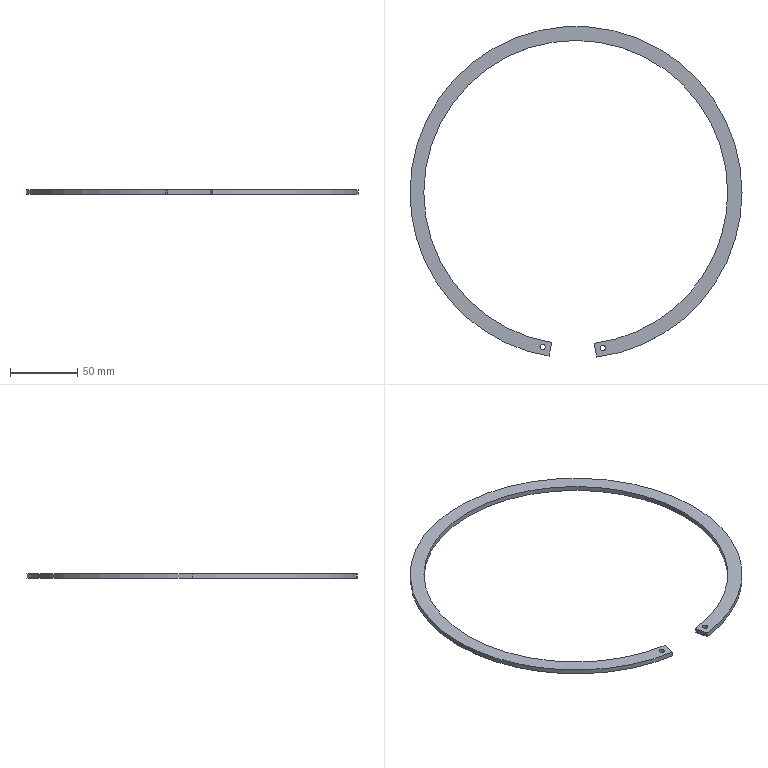Part | STEP file | Expansion ring | 1 solid | 14 faces | box 245.982 x 245.031 x 3.5 mm | volume 25663 mm3 | cylinder 10 | plane 4 | commonest cylinder face diameters 3.966 x4 225.162 x3 245.982 x3
STEP:
#1=CARTESIAN_POINT('',(0.,0.,0.));
#2=DIRECTION('',(0.,0.,1.));
#3=DIRECTION('',(1.,0.,0.));
#4=AXIS2_PLACEMENT_3D('',#1,#2,#3);
#5=CARTESIAN_POINT('',(-24.239,-114.472,3.5));
#6=VERTEX_POINT('',#5);
#7=CARTESIAN_POINT('',(-24.239,-114.472,0.));
#8=VERTEX_POINT('',#7);
#9=CARTESIAN_POINT('',(-24.239,-114.472,3.5));
#10=DIRECTION('',(0.,0.,-1.));
#11=VECTOR('',#10,1.);
#12=LINE('',#9,#11);
#13=CARTESIAN_POINT('',(-22.256,-114.472,3.5));
#14=DIRECTION('',(0.,0.,-1.));
#15=DIRECTION('',(-1.,0.,0.));
#16=AXIS2_PLACEMENT_3D('',#13,#14,#15);
#17=CYLINDRICAL_SURFACE('',#16,1.983);
#18=CARTESIAN_POINT('',(6.283,0.));
#19=DIRECTION('',(0.,1.));
#20=VECTOR('',#19,1.);
#21=LINE('',#18,#20);
#22=(GEOMETRIC_REPRESENTATION_CONTEXT(2)PARAMETRIC_REPRESENTATION_CONTEXT()REPRESENTATION_CONTEXT('',''));
#23=DEFINITIONAL_REPRESENTATION('',(#21),#22);
#24=PCURVE('',#17,#23);
#25=CARTESIAN_POINT('',(-22.256,-114.472,3.5));
#26=DIRECTION('',(0.,0.,-1.));
#27=DIRECTION('',(-1.,0.,0.));
#28=AXIS2_PLACEMENT_3D('',#25,#26,#27);
#29=CYLINDRICAL_SURFACE('',#28,1.983);
#30=CARTESIAN_POINT('',(0.,0.));
#31=DIRECTION('',(0.,1.));
#32=VECTOR('',#31,1.);
#33=LINE('',#30,#32);
#34=(GEOMETRIC_REPRESENTATION_CONTEXT(2)PARAMETRIC_REPRESENTATION_CONTEXT()REPRESENTATION_CONTEXT('',''));
#35=DEFINITIONAL_REPRESENTATION('',(#33),#34);
#36=PCURVE('',#29,#35);
#37=SURFACE_CURVE('',#12,(#24,#36),.PCURVE_S1.);
#38=EDGE_CURVE('',#6,#8,#37,.T.);
#39=ORIENTED_EDGE('',*,*,#38,.T.);
#40=CARTESIAN_POINT('',(-20.273,-114.472,0.));
#41=VERTEX_POINT('',#40);
#42=CARTESIAN_POINT('',(-22.256,-114.472,0.));
#43=DIRECTION('',(0.,0.,1.));
#44=DIRECTION('',(1.,0.,0.));
#45=AXIS2_PLACEMENT_3D('',#42,#43,#44);
#46=CIRCLE('',#45,1.983);
#47=CARTESIAN_POINT('',(9.425,3.5));
#48=DIRECTION('',(-1.,0.));
#49=VECTOR('',#48,1.);
#50=LINE('',#47,#49);
#51=(GEOMETRIC_REPRESENTATION_CONTEXT(2)PARAMETRIC_REPRESENTATION_CONTEXT()REPRESENTATION_CONTEXT('',''));
#52=DEFINITIONAL_REPRESENTATION('',(#50),#51);
#53=PCURVE('',#17,#52);
#54=CARTESIAN_POINT('',(2.29,-0.01991,0.));
#55=DIRECTION('',(0.,0.,1.));
#56=DIRECTION('',(1.,0.,0.));
#57=AXIS2_PLACEMENT_3D('',#54,#55,#56);
#58=PLANE('',#57);
#59=CARTESIAN_POINT('',(-24.546,-114.452));
#60=DIRECTION('',(1.,0.));
#61=AXIS2_PLACEMENT_2D('',#59,#60);
#62=CIRCLE('',#61,1.983);
#63=(GEOMETRIC_REPRESENTATION_CONTEXT(2)PARAMETRIC_REPRESENTATION_CONTEXT()REPRESENTATION_CONTEXT('',''));
#64=DEFINITIONAL_REPRESENTATION('',(#62),#63);
#65=PCURVE('',#58,#64);
#66=SURFACE_CURVE('',#46,(#53,#65),.PCURVE_S1.);
#67=EDGE_CURVE('',#8,#41,#66,.T.);
#68=ORIENTED_EDGE('',*,*,#67,.T.);
#69=CARTESIAN_POINT('',(-20.273,-114.472,3.5));
#70=VERTEX_POINT('',#69);
#71=CARTESIAN_POINT('',(-20.273,-114.472,3.5));
#72=DIRECTION('',(0.,0.,-1.));
#73=VECTOR('',#72,1.);
#74=LINE('',#71,#73);
#75=CARTESIAN_POINT('',(3.142,0.));
#76=DIRECTION('',(0.,1.));
#77=VECTOR('',#76,1.);
#78=LINE('',#75,#77);
#79=(GEOMETRIC_REPRESENTATION_CONTEXT(2)PARAMETRIC_REPRESENTATION_CONTEXT()REPRESENTATION_CONTEXT('',''));
#80=DEFINITIONAL_REPRESENTATION('',(#78),#79);
#81=PCURVE('',#17,#80);
#82=CARTESIAN_POINT('',(3.142,0.));
#83=DIRECTION('',(0.,1.));
#84=VECTOR('',#83,1.);
#85=LINE('',#82,#84);
#86=(GEOMETRIC_REPRESENTATION_CONTEXT(2)PARAMETRIC_REPRESENTATION_CONTEXT()REPRESENTATION_CONTEXT('',''));
#87=DEFINITIONAL_REPRESENTATION('',(#85),#86);
#88=PCURVE('',#29,#87);
#89=SURFACE_CURVE('',#74,(#81,#88),.PCURVE_S1.);
#90=EDGE_CURVE('',#70,#41,#89,.T.);
#91=ORIENTED_EDGE('',*,*,#90,.F.);
#92=CARTESIAN_POINT('',(-22.256,-114.472,3.5));
#93=DIRECTION('',(0.,0.,1.));
#94=DIRECTION('',(1.,0.,0.));
#95=AXIS2_PLACEMENT_3D('',#92,#93,#94);
#96=CIRCLE('',#95,1.983);
#97=CARTESIAN_POINT('',(9.425,0.));
#98=DIRECTION('',(-1.,0.));
#99=VECTOR('',#98,1.);
#100=LINE('',#97,#99);
#101=(GEOMETRIC_REPRESENTATION_CONTEXT(2)PARAMETRIC_REPRESENTATION_CONTEXT()REPRESENTATION_CONTEXT('',''));
#102=DEFINITIONAL_REPRESENTATION('',(#100),#101);
#103=PCURVE('',#17,#102);
#104=CARTESIAN_POINT('',(2.29,-0.01991,3.5));
#105=DIRECTION('',(0.,0.,1.));
#106=DIRECTION('',(1.,0.,0.));
#107=AXIS2_PLACEMENT_3D('',#104,#105,#106);
#108=PLANE('',#107);
#109=CARTESIAN_POINT('',(-24.546,-114.452));
#110=DIRECTION('',(1.,0.));
#111=AXIS2_PLACEMENT_2D('',#109,#110);
#112=CIRCLE('',#111,1.983);
#113=(GEOMETRIC_REPRESENTATION_CONTEXT(2)PARAMETRIC_REPRESENTATION_CONTEXT()REPRESENTATION_CONTEXT('',''));
#114=DEFINITIONAL_REPRESENTATION('',(#112),#113);
#115=PCURVE('',#108,#114);
#116=SURFACE_CURVE('',#96,(#103,#115),.PCURVE_S1.);
#117=EDGE_CURVE('',#6,#70,#116,.T.);
#118=ORIENTED_EDGE('',*,*,#117,.F.);
#119=EDGE_LOOP('',(#39,#68,#91,#118));
#120=FACE_BOUND('',#119,.F.);
#121=ADVANCED_FACE('',(#120),#17,.F.);
#122=CARTESIAN_POINT('',(20.369,-115.146,3.5));
#123=VERTEX_POINT('',#122);
#124=CARTESIAN_POINT('',(20.369,-115.146,0.));
#125=VERTEX_POINT('',#124);
#126=CARTESIAN_POINT('',(20.369,-115.146,3.5));
#127=DIRECTION('',(0.,0.,-1.));
#128=VECTOR('',#127,1.);
#129=LINE('',#126,#128);
#130=CARTESIAN_POINT('',(22.352,-115.146,3.5));
#131=DIRECTION('',(0.,0.,-1.));
#132=DIRECTION('',(-1.,0.,0.));
#133=AXIS2_PLACEMENT_3D('',#130,#131,#132);
#134=CYLINDRICAL_SURFACE('',#133,1.983);
#135=CARTESIAN_POINT('',(6.283,0.));
#136=DIRECTION('',(0.,1.));
#137=VECTOR('',#136,1.);
#138=LINE('',#135,#137);
#139=(GEOMETRIC_REPRESENTATION_CONTEXT(2)PARAMETRIC_REPRESENTATION_CONTEXT()REPRESENTATION_CONTEXT('',''));
#140=DEFINITIONAL_REPRESENTATION('',(#138),#139);
#141=PCURVE('',#134,#140);
#142=CARTESIAN_POINT('',(22.352,-115.146,3.5));
#143=DIRECTION('',(0.,0.,-1.));
#144=DIRECTION('',(-1.,0.,0.));
#145=AXIS2_PLACEMENT_3D('',#142,#143,#144);
#146=CYLINDRICAL_SURFACE('',#145,1.983);
#147=CARTESIAN_POINT('',(0.,0.));
#148=DIRECTION('',(0.,1.));
#149=VECTOR('',#148,1.);
#150=LINE('',#147,#149);
#151=(GEOMETRIC_REPRESENTATION_CONTEXT(2)PARAMETRIC_REPRESENTATION_CONTEXT()REPRESENTATION_CONTEXT('',''));
#152=DEFINITIONAL_REPRESENTATION('',(#150),#151);
#153=PCURVE('',#146,#152);
#154=SURFACE_CURVE('',#129,(#141,#153),.PCURVE_S1.);
#155=EDGE_CURVE('',#123,#125,#154,.T.);
#156=ORIENTED_EDGE('',*,*,#155,.T.);
#157=CARTESIAN_POINT('',(24.335,-115.146,0.));
#158=VERTEX_POINT('',#157);
#159=CARTESIAN_POINT('',(22.352,-115.146,0.));
#160=DIRECTION('',(0.,0.,1.));
#161=DIRECTION('',(1.,0.,0.));
#162=AXIS2_PLACEMENT_3D('',#159,#160,#161);
#163=CIRCLE('',#162,1.983);
#164=CARTESIAN_POINT('',(9.425,3.5));
#165=DIRECTION('',(-1.,0.));
#166=VECTOR('',#165,1.);
#167=LINE('',#164,#166);
#168=(GEOMETRIC_REPRESENTATION_CONTEXT(2)PARAMETRIC_REPRESENTATION_CONTEXT()REPRESENTATION_CONTEXT('',''));
#169=DEFINITIONAL_REPRESENTATION('',(#167),#168);
#170=PCURVE('',#134,#169);
#171=CARTESIAN_POINT('',(20.062,-115.126));
#172=DIRECTION('',(1.,0.));
#173=AXIS2_PLACEMENT_2D('',#171,#172);
#174=CIRCLE('',#173,1.983);
#175=(GEOMETRIC_REPRESENTATION_CONTEXT(2)PARAMETRIC_REPRESENTATION_CONTEXT()REPRESENTATION_CONTEXT('',''));
#176=DEFINITIONAL_REPRESENTATION('',(#174),#175);
#177=PCURVE('',#58,#176);
#178=SURFACE_CURVE('',#163,(#170,#177),.PCURVE_S1.);
#179=EDGE_CURVE('',#125,#158,#178,.T.);
#180=ORIENTED_EDGE('',*,*,#179,.T.);
#181=CARTESIAN_POINT('',(24.335,-115.146,3.5));
#182=VERTEX_POINT('',#181);
#183=CARTESIAN_POINT('',(24.335,-115.146,3.5));
#184=DIRECTION('',(0.,0.,-1.));
#185=VECTOR('',#184,1.);
#186=LINE('',#183,#185);
#187=CARTESIAN_POINT('',(3.142,0.));
#188=DIRECTION('',(0.,1.));
#189=VECTOR('',#188,1.);
#190=LINE('',#187,#189);
#191=(GEOMETRIC_REPRESENTATION_CONTEXT(2)PARAMETRIC_REPRESENTATION_CONTEXT()REPRESENTATION_CONTEXT('',''));
#192=DEFINITIONAL_REPRESENTATION('',(#190),#191);
#193=PCURVE('',#134,#192);
#194=CARTESIAN_POINT('',(3.142,0.));
#195=DIRECTION('',(0.,1.));
#196=VECTOR('',#195,1.);
#197=LINE('',#194,#196);
#198=(GEOMETRIC_REPRESENTATION_CONTEXT(2)PARAMETRIC_REPRESENTATION_CONTEXT()REPRESENTATION_CONTEXT('',''));
#199=DEFINITIONAL_REPRESENTATION('',(#197),#198);
#200=PCURVE('',#146,#199);
#201=SURFACE_CURVE('',#186,(#193,#200),.PCURVE_S1.);
#202=EDGE_CURVE('',#182,#158,#201,.T.);
#203=ORIENTED_EDGE('',*,*,#202,.F.);
#204=CARTESIAN_POINT('',(22.352,-115.146,3.5));
#205=DIRECTION('',(0.,0.,1.));
#206=DIRECTION('',(1.,0.,0.));
#207=AXIS2_PLACEMENT_3D('',#204,#205,#206);
#208=CIRCLE('',#207,1.983);
#209=CARTESIAN_POINT('',(9.425,0.));
#210=DIRECTION('',(-1.,0.));
#211=VECTOR('',#210,1.);
#212=LINE('',#209,#211);
#213=(GEOMETRIC_REPRESENTATION_CONTEXT(2)PARAMETRIC_REPRESENTATION_CONTEXT()REPRESENTATION_CONTEXT('',''));
#214=DEFINITIONAL_REPRESENTATION('',(#212),#213);
#215=PCURVE('',#134,#214);
#216=CARTESIAN_POINT('',(20.062,-115.126));
#217=DIRECTION('',(1.,0.));
#218=AXIS2_PLACEMENT_2D('',#216,#217);
#219=CIRCLE('',#218,1.983);
#220=(GEOMETRIC_REPRESENTATION_CONTEXT(2)PARAMETRIC_REPRESENTATION_CONTEXT()REPRESENTATION_CONTEXT('',''));
#221=DEFINITIONAL_REPRESENTATION('',(#219),#220);
#222=PCURVE('',#108,#221);
#223=SURFACE_CURVE('',#208,(#215,#222),.PCURVE_S1.);
#224=EDGE_CURVE('',#123,#182,#223,.T.);
#225=ORIENTED_EDGE('',*,*,#224,.F.);
#226=EDGE_LOOP('',(#156,#180,#203,#225));
#227=FACE_BOUND('',#226,.F.);
#228=ADVANCED_FACE('',(#227),#134,.F.);
#229=CARTESIAN_POINT('',(125.475,-0.001316,3.5));
#230=VERTEX_POINT('',#229);
#231=CARTESIAN_POINT('',(-120.508,-0.001316,3.5));
#232=VERTEX_POINT('',#231);
#233=CARTESIAN_POINT('',(2.483,-0.001316,3.5));
#234=DIRECTION('',(0.,0.,1.));
#235=DIRECTION('',(1.,0.,0.));
#236=AXIS2_PLACEMENT_3D('',#233,#234,#235);
#237=CIRCLE('',#236,122.991);
#238=CARTESIAN_POINT('',(2.483,-0.001316,3.5));
#239=DIRECTION('',(0.,0.,-1.));
#240=DIRECTION('',(-1.,0.,0.));
#241=AXIS2_PLACEMENT_3D('',#238,#239,#240);
#242=CYLINDRICAL_SURFACE('',#241,122.991);
#243=CARTESIAN_POINT('',(3.142,0.));
#244=DIRECTION('',(-1.,0.));
#245=VECTOR('',#244,1.);
#246=LINE('',#243,#245);
#247=(GEOMETRIC_REPRESENTATION_CONTEXT(2)PARAMETRIC_REPRESENTATION_CONTEXT()REPRESENTATION_CONTEXT('',''));
#248=DEFINITIONAL_REPRESENTATION('',(#246),#247);
#249=PCURVE('',#242,#248);
#250=CARTESIAN_POINT('',(0.1933,0.01859));
#251=DIRECTION('',(1.,0.));
#252=AXIS2_PLACEMENT_2D('',#250,#251);
#253=CIRCLE('',#252,122.991);
#254=(GEOMETRIC_REPRESENTATION_CONTEXT(2)PARAMETRIC_REPRESENTATION_CONTEXT()REPRESENTATION_CONTEXT('',''));
#255=DEFINITIONAL_REPRESENTATION('',(#253),#254);
#256=PCURVE('',#108,#255);
#257=SURFACE_CURVE('',#237,(#249,#256),.PCURVE_S1.);
#258=EDGE_CURVE('',#230,#232,#257,.T.);
#259=ORIENTED_EDGE('',*,*,#258,.F.);
#260=CARTESIAN_POINT('',(125.475,-0.001316,0.));
#261=VERTEX_POINT('',#260);
#262=CARTESIAN_POINT('',(125.475,-0.001316,3.5));
#263=DIRECTION('',(0.,0.,-1.));
#264=VECTOR('',#263,1.);
#265=LINE('',#262,#264);
#266=CARTESIAN_POINT('',(3.142,0.));
#267=DIRECTION('',(0.,1.));
#268=VECTOR('',#267,1.);
#269=LINE('',#266,#268);
#270=(GEOMETRIC_REPRESENTATION_CONTEXT(2)PARAMETRIC_REPRESENTATION_CONTEXT()REPRESENTATION_CONTEXT('',''));
#271=DEFINITIONAL_REPRESENTATION('',(#269),#270);
#272=PCURVE('',#242,#271);
#273=CARTESIAN_POINT('',(2.483,-0.001316,3.5));
#274=DIRECTION('',(0.,0.,-1.));
#275=DIRECTION('',(-1.,0.,0.));
#276=AXIS2_PLACEMENT_3D('',#273,#274,#275);
#277=CYLINDRICAL_SURFACE('',#276,122.991);
#278=CARTESIAN_POINT('',(3.142,0.));
#279=DIRECTION('',(0.,1.));
#280=VECTOR('',#279,1.);
#281=LINE('',#278,#280);
#282=(GEOMETRIC_REPRESENTATION_CONTEXT(2)PARAMETRIC_REPRESENTATION_CONTEXT()REPRESENTATION_CONTEXT('',''));
#283=DEFINITIONAL_REPRESENTATION('',(#281),#282);
#284=PCURVE('',#277,#283);
#285=SURFACE_CURVE('',#265,(#272,#284),.PCURVE_S1.);
#286=EDGE_CURVE('',#230,#261,#285,.T.);
#287=ORIENTED_EDGE('',*,*,#286,.T.);
#288=CARTESIAN_POINT('',(-120.508,-0.001316,0.));
#289=VERTEX_POINT('',#288);
#290=CARTESIAN_POINT('',(2.483,-0.001316,0.));
#291=DIRECTION('',(0.,0.,1.));
#292=DIRECTION('',(1.,0.,0.));
#293=AXIS2_PLACEMENT_3D('',#290,#291,#292);
#294=CIRCLE('',#293,122.991);
#295=CARTESIAN_POINT('',(3.142,3.5));
#296=DIRECTION('',(-1.,0.));
#297=VECTOR('',#296,1.);
#298=LINE('',#295,#297);
#299=(GEOMETRIC_REPRESENTATION_CONTEXT(2)PARAMETRIC_REPRESENTATION_CONTEXT()REPRESENTATION_CONTEXT('',''));
#300=DEFINITIONAL_REPRESENTATION('',(#298),#299);
#301=PCURVE('',#242,#300);
#302=CARTESIAN_POINT('',(0.1933,0.01859));
#303=DIRECTION('',(1.,0.));
#304=AXIS2_PLACEMENT_2D('',#302,#303);
#305=CIRCLE('',#304,122.991);
#306=(GEOMETRIC_REPRESENTATION_CONTEXT(2)PARAMETRIC_REPRESENTATION_CONTEXT()REPRESENTATION_CONTEXT('',''));
#307=DEFINITIONAL_REPRESENTATION('',(#305),#306);
#308=PCURVE('',#58,#307);
#309=SURFACE_CURVE('',#294,(#301,#308),.PCURVE_S1.);
#310=EDGE_CURVE('',#261,#289,#309,.T.);
#311=ORIENTED_EDGE('',*,*,#310,.T.);
#312=CARTESIAN_POINT('',(-120.508,-0.001316,3.5));
#313=DIRECTION('',(0.,0.,-1.));
#314=VECTOR('',#313,1.);
#315=LINE('',#312,#314);
#316=CARTESIAN_POINT('',(0.,0.));
#317=DIRECTION('',(0.,1.));
#318=VECTOR('',#317,1.);
#319=LINE('',#316,#318);
#320=(GEOMETRIC_REPRESENTATION_CONTEXT(2)PARAMETRIC_REPRESENTATION_CONTEXT()REPRESENTATION_CONTEXT('',''));
#321=DEFINITIONAL_REPRESENTATION('',(#319),#320);
#322=PCURVE('',#242,#321);
#323=CARTESIAN_POINT('',(2.483,-0.001316,3.5));
#324=DIRECTION('',(0.,0.,-1.));
#325=DIRECTION('',(-1.,0.,0.));
#326=AXIS2_PLACEMENT_3D('',#323,#324,#325);
#327=CYLINDRICAL_SURFACE('',#326,122.991);
#328=CARTESIAN_POINT('',(6.283,0.));
#329=DIRECTION('',(0.,1.));
#330=VECTOR('',#329,1.);
#331=LINE('',#328,#330);
#332=(GEOMETRIC_REPRESENTATION_CONTEXT(2)PARAMETRIC_REPRESENTATION_CONTEXT()REPRESENTATION_CONTEXT('',''));
#333=DEFINITIONAL_REPRESENTATION('',(#331),#332);
#334=PCURVE('',#327,#333);
#335=SURFACE_CURVE('',#315,(#322,#334),.PCURVE_S1.);
#336=EDGE_CURVE('',#232,#289,#335,.T.);
#337=ORIENTED_EDGE('',*,*,#336,.F.);
#338=EDGE_LOOP('',(#259,#287,#311,#337));
#339=FACE_BOUND('',#338,.T.);
#340=ADVANCED_FACE('',(#339),#242,.T.);
#341=CARTESIAN_POINT('',(-17.517,-121.355,3.5));
#342=VERTEX_POINT('',#341);
#343=CARTESIAN_POINT('',(2.483,-0.001316,3.5));
#344=DIRECTION('',(0.,0.,1.));
#345=DIRECTION('',(1.,0.,0.));
#346=AXIS2_PLACEMENT_3D('',#343,#344,#345);
#347=CIRCLE('',#346,122.991);
#348=CARTESIAN_POINT('',(9.425,0.));
#349=DIRECTION('',(-1.,0.));
#350=VECTOR('',#349,1.);
#351=LINE('',#348,#350);
#352=(GEOMETRIC_REPRESENTATION_CONTEXT(2)PARAMETRIC_REPRESENTATION_CONTEXT()REPRESENTATION_CONTEXT('',''));
#353=DEFINITIONAL_REPRESENTATION('',(#351),#352);
#354=PCURVE('',#327,#353);
#355=CARTESIAN_POINT('',(0.1933,0.01859));
#356=DIRECTION('',(1.,0.));
#357=AXIS2_PLACEMENT_2D('',#355,#356);
#358=CIRCLE('',#357,122.991);
#359=(GEOMETRIC_REPRESENTATION_CONTEXT(2)PARAMETRIC_REPRESENTATION_CONTEXT()REPRESENTATION_CONTEXT('',''));
#360=DEFINITIONAL_REPRESENTATION('',(#358),#359);
#361=PCURVE('',#108,#360);
#362=SURFACE_CURVE('',#347,(#354,#361),.PCURVE_S1.);
#363=EDGE_CURVE('',#232,#342,#362,.T.);
#364=ORIENTED_EDGE('',*,*,#363,.F.);
#365=ORIENTED_EDGE('',*,*,#336,.T.);
#366=CARTESIAN_POINT('',(-17.517,-121.355,0.));
#367=VERTEX_POINT('',#366);
#368=CARTESIAN_POINT('',(2.483,-0.001316,0.));
#369=DIRECTION('',(0.,0.,1.));
#370=DIRECTION('',(1.,0.,0.));
#371=AXIS2_PLACEMENT_3D('',#368,#369,#370);
#372=CIRCLE('',#371,122.991);
#373=CARTESIAN_POINT('',(9.425,3.5));
#374=DIRECTION('',(-1.,0.));
#375=VECTOR('',#374,1.);
#376=LINE('',#373,#375);
#377=(GEOMETRIC_REPRESENTATION_CONTEXT(2)PARAMETRIC_REPRESENTATION_CONTEXT()REPRESENTATION_CONTEXT('',''));
#378=DEFINITIONAL_REPRESENTATION('',(#376),#377);
#379=PCURVE('',#327,#378);
#380=CARTESIAN_POINT('',(0.1933,0.01859));
#381=DIRECTION('',(1.,0.));
#382=AXIS2_PLACEMENT_2D('',#380,#381);
#383=CIRCLE('',#382,122.991);
#384=(GEOMETRIC_REPRESENTATION_CONTEXT(2)PARAMETRIC_REPRESENTATION_CONTEXT()REPRESENTATION_CONTEXT('',''));
#385=DEFINITIONAL_REPRESENTATION('',(#383),#384);
#386=PCURVE('',#58,#385);
#387=SURFACE_CURVE('',#372,(#379,#386),.PCURVE_S1.);
#388=EDGE_CURVE('',#289,#367,#387,.T.);
#389=ORIENTED_EDGE('',*,*,#388,.T.);
#390=CARTESIAN_POINT('',(-17.517,-121.355,3.5));
#391=DIRECTION('',(0.,0.,-1.));
#392=VECTOR('',#391,1.);
#393=LINE('',#390,#392);
#394=CARTESIAN_POINT('',(4.876,0.));
#395=DIRECTION('',(0.,1.));
#396=VECTOR('',#395,1.);
#397=LINE('',#394,#396);
#398=(GEOMETRIC_REPRESENTATION_CONTEXT(2)PARAMETRIC_REPRESENTATION_CONTEXT()REPRESENTATION_CONTEXT('',''));
#399=DEFINITIONAL_REPRESENTATION('',(#397),#398);
#400=PCURVE('',#327,#399);
#401=CARTESIAN_POINT('',(-15.505,-111.186,3.5));
#402=DIRECTION('',(-0.981,0.1941,0.));
#403=DIRECTION('',(-0.1941,-0.981,0.));
#404=AXIS2_PLACEMENT_3D('',#401,#402,#403);
#405=PLANE('',#404);
#406=CARTESIAN_POINT('',(10.367,0.));
#407=DIRECTION('',(0.,-1.));
#408=VECTOR('',#407,1.);
#409=LINE('',#406,#408);
#410=(GEOMETRIC_REPRESENTATION_CONTEXT(2)PARAMETRIC_REPRESENTATION_CONTEXT()REPRESENTATION_CONTEXT('',''));
#411=DEFINITIONAL_REPRESENTATION('',(#409),#410);
#412=PCURVE('',#405,#411);
#413=SURFACE_CURVE('',#393,(#400,#412),.PCURVE_S1.);
#414=EDGE_CURVE('',#342,#367,#413,.T.);
#415=ORIENTED_EDGE('',*,*,#414,.F.);
#416=EDGE_LOOP('',(#364,#365,#389,#415));
#417=FACE_BOUND('',#416,.T.);
#418=ADVANCED_FACE('',(#417),#327,.T.);
#419=CARTESIAN_POINT('',(15.865,-111.78,3.5));
#420=VERTEX_POINT('',#419);
#421=CARTESIAN_POINT('',(15.865,-111.78,0.));
#422=VERTEX_POINT('',#421);
#423=CARTESIAN_POINT('',(15.865,-111.78,3.5));
#424=DIRECTION('',(0.,0.,-1.));
#425=VECTOR('',#424,1.);
#426=LINE('',#423,#425);
#427=CARTESIAN_POINT('',(2.29,-0.01991,3.5));
#428=DIRECTION('',(0.,0.,-1.));
#429=DIRECTION('',(-1.,0.,0.));
#430=AXIS2_PLACEMENT_3D('',#427,#428,#429);
#431=CYLINDRICAL_SURFACE('',#430,112.581);
#432=CARTESIAN_POINT('',(4.592,0.));
#433=DIRECTION('',(0.,1.));
#434=VECTOR('',#433,1.);
#435=LINE('',#432,#434);
#436=(GEOMETRIC_REPRESENTATION_CONTEXT(2)PARAMETRIC_REPRESENTATION_CONTEXT()REPRESENTATION_CONTEXT('',''));
#437=DEFINITIONAL_REPRESENTATION('',(#435),#436);
#438=PCURVE('',#431,#437);
#439=CARTESIAN_POINT('',(15.865,-111.78,3.5));
#440=DIRECTION('',(0.9835,0.1812,0.));
#441=DIRECTION('',(-0.1812,0.9835,0.));
#442=AXIS2_PLACEMENT_3D('',#439,#440,#441);
#443=PLANE('',#442);
#444=CARTESIAN_POINT('',(0.,0.));
#445=DIRECTION('',(0.,-1.));
#446=VECTOR('',#445,1.);
#447=LINE('',#444,#446);
#448=(GEOMETRIC_REPRESENTATION_CONTEXT(2)PARAMETRIC_REPRESENTATION_CONTEXT()REPRESENTATION_CONTEXT('',''));
#449=DEFINITIONAL_REPRESENTATION('',(#447),#448);
#450=PCURVE('',#443,#449);
#451=SURFACE_CURVE('',#426,(#438,#450),.PCURVE_S1.);
#452=EDGE_CURVE('',#420,#422,#451,.T.);
#453=ORIENTED_EDGE('',*,*,#452,.T.);
#454=CARTESIAN_POINT('',(114.871,-0.01991,0.));
#455=VERTEX_POINT('',#454);
#456=CARTESIAN_POINT('',(2.29,-0.01991,0.));
#457=DIRECTION('',(0.,0.,-1.));
#458=DIRECTION('',(1.,0.,0.));
#459=AXIS2_PLACEMENT_3D('',#456,#457,#458);
#460=CIRCLE('',#459,112.581);
#461=CARTESIAN_POINT('',(3.142,3.5));
#462=DIRECTION('',(1.,0.));
#463=VECTOR('',#462,1.);
#464=LINE('',#461,#463);
#465=(GEOMETRIC_REPRESENTATION_CONTEXT(2)PARAMETRIC_REPRESENTATION_CONTEXT()REPRESENTATION_CONTEXT('',''));
#466=DEFINITIONAL_REPRESENTATION('',(#464),#465);
#467=PCURVE('',#431,#466);
#468=CARTESIAN_POINT('',(112.581,0.));
#469=CARTESIAN_POINT('',(112.581,-194.996));
#470=CARTESIAN_POINT('',(-56.291,-97.498));
#471=CARTESIAN_POINT('',(-225.162,0.));
#472=CARTESIAN_POINT('',(-56.291,97.498));
#473=CARTESIAN_POINT('',(112.581,194.996));
#474=CARTESIAN_POINT('',(112.581,0.));
#475=(BOUNDED_CURVE()B_SPLINE_CURVE(2,(#468,#469,#470,#471,#472,#473,#474),.UNSPECIFIED.,.T.,.F.)B_SPLINE_CURVE_WITH_KNOTS((1,2,2,2,2,1),(-2.094,0.,2.094,4.189,6.283,8.378),.UNSPECIFIED.)CURVE()GEOMETRIC_REPRESENTATION_ITEM()RATIONAL_B_SPLINE_CURVE((1.,0.5,1.,0.5,1.,0.5,1.))REPRESENTATION_ITEM(''));
#476=(GEOMETRIC_REPRESENTATION_CONTEXT(2)PARAMETRIC_REPRESENTATION_CONTEXT()REPRESENTATION_CONTEXT('',''));
#477=DEFINITIONAL_REPRESENTATION('',(#475),#476);
#478=PCURVE('',#58,#477);
#479=SURFACE_CURVE('',#460,(#467,#478),.PCURVE_S1.);
#480=EDGE_CURVE('',#455,#422,#479,.T.);
#481=ORIENTED_EDGE('',*,*,#480,.F.);
#482=CARTESIAN_POINT('',(114.871,-0.01991,3.5));
#483=VERTEX_POINT('',#482);
#484=CARTESIAN_POINT('',(114.871,-0.01991,3.5));
#485=DIRECTION('',(0.,0.,-1.));
#486=VECTOR('',#485,1.);
#487=LINE('',#484,#486);
#488=CARTESIAN_POINT('',(3.142,0.));
#489=DIRECTION('',(0.,1.));
#490=VECTOR('',#489,1.);
#491=LINE('',#488,#490);
#492=(GEOMETRIC_REPRESENTATION_CONTEXT(2)PARAMETRIC_REPRESENTATION_CONTEXT()REPRESENTATION_CONTEXT('',''));
#493=DEFINITIONAL_REPRESENTATION('',(#491),#492);
#494=PCURVE('',#431,#493);
#495=CARTESIAN_POINT('',(2.29,-0.01991,3.5));
#496=DIRECTION('',(0.,0.,-1.));
#497=DIRECTION('',(-1.,0.,0.));
#498=AXIS2_PLACEMENT_3D('',#495,#496,#497);
#499=CYLINDRICAL_SURFACE('',#498,112.581);
#500=CARTESIAN_POINT('',(3.142,0.));
#501=DIRECTION('',(0.,1.));
#502=VECTOR('',#501,1.);
#503=LINE('',#500,#502);
#504=(GEOMETRIC_REPRESENTATION_CONTEXT(2)PARAMETRIC_REPRESENTATION_CONTEXT()REPRESENTATION_CONTEXT('',''));
#505=DEFINITIONAL_REPRESENTATION('',(#503),#504);
#506=PCURVE('',#499,#505);
#507=SURFACE_CURVE('',#487,(#494,#506),.PCURVE_S1.);
#508=EDGE_CURVE('',#483,#455,#507,.T.);
#509=ORIENTED_EDGE('',*,*,#508,.F.);
#510=CARTESIAN_POINT('',(2.29,-0.01991,3.5));
#511=DIRECTION('',(0.,0.,-1.));
#512=DIRECTION('',(1.,0.,0.));
#513=AXIS2_PLACEMENT_3D('',#510,#511,#512);
#514=CIRCLE('',#513,112.581);
#515=CARTESIAN_POINT('',(3.142,0.));
#516=DIRECTION('',(1.,0.));
#517=VECTOR('',#516,1.);
#518=LINE('',#515,#517);
#519=(GEOMETRIC_REPRESENTATION_CONTEXT(2)PARAMETRIC_REPRESENTATION_CONTEXT()REPRESENTATION_CONTEXT('',''));
#520=DEFINITIONAL_REPRESENTATION('',(#518),#519);
#521=PCURVE('',#431,#520);
#522=CARTESIAN_POINT('',(112.581,0.));
#523=CARTESIAN_POINT('',(112.581,-194.996));
#524=CARTESIAN_POINT('',(-56.291,-97.498));
#525=CARTESIAN_POINT('',(-225.162,0.));
#526=CARTESIAN_POINT('',(-56.291,97.498));
#527=CARTESIAN_POINT('',(112.581,194.996));
#528=CARTESIAN_POINT('',(112.581,0.));
#529=(BOUNDED_CURVE()B_SPLINE_CURVE(2,(#522,#523,#524,#525,#526,#527,#528),.UNSPECIFIED.,.T.,.F.)B_SPLINE_CURVE_WITH_KNOTS((1,2,2,2,2,1),(-2.094,0.,2.094,4.189,6.283,8.378),.UNSPECIFIED.)CURVE()GEOMETRIC_REPRESENTATION_ITEM()RATIONAL_B_SPLINE_CURVE((1.,0.5,1.,0.5,1.,0.5,1.))REPRESENTATION_ITEM(''));
#530=(GEOMETRIC_REPRESENTATION_CONTEXT(2)PARAMETRIC_REPRESENTATION_CONTEXT()REPRESENTATION_CONTEXT('',''));
#531=DEFINITIONAL_REPRESENTATION('',(#529),#530);
#532=PCURVE('',#108,#531);
#533=SURFACE_CURVE('',#514,(#521,#532),.PCURVE_S1.);
#534=EDGE_CURVE('',#483,#420,#533,.T.);
#535=ORIENTED_EDGE('',*,*,#534,.T.);
#536=EDGE_LOOP('',(#453,#481,#509,#535));
#537=FACE_BOUND('',#536,.F.);
#538=ADVANCED_FACE('',(#537),#431,.F.);
#539=CARTESIAN_POINT('',(-110.291,-0.01991,0.));
#540=VERTEX_POINT('',#539);
#541=CARTESIAN_POINT('',(2.29,-0.01991,0.));
#542=DIRECTION('',(0.,0.,-1.));
#543=DIRECTION('',(1.,0.,0.));
#544=AXIS2_PLACEMENT_3D('',#541,#542,#543);
#545=CIRCLE('',#544,112.581);
#546=CARTESIAN_POINT('',(-3.142,3.5));
#547=DIRECTION('',(1.,0.));
#548=VECTOR('',#547,1.);
#549=LINE('',#546,#548);
#550=(GEOMETRIC_REPRESENTATION_CONTEXT(2)PARAMETRIC_REPRESENTATION_CONTEXT()REPRESENTATION_CONTEXT('',''));
#551=DEFINITIONAL_REPRESENTATION('',(#549),#550);
#552=PCURVE('',#499,#551);
#553=CARTESIAN_POINT('',(112.581,0.));
#554=CARTESIAN_POINT('',(112.581,-194.996));
#555=CARTESIAN_POINT('',(-56.291,-97.498));
#556=CARTESIAN_POINT('',(-225.162,0.));
#557=CARTESIAN_POINT('',(-56.291,97.498));
#558=CARTESIAN_POINT('',(112.581,194.996));
#559=CARTESIAN_POINT('',(112.581,0.));
#560=(BOUNDED_CURVE()B_SPLINE_CURVE(2,(#553,#554,#555,#556,#557,#558,#559),.UNSPECIFIED.,.T.,.F.)B_SPLINE_CURVE_WITH_KNOTS((1,2,2,2,2,1),(-2.094,0.,2.094,4.189,6.283,8.378),.UNSPECIFIED.)CURVE()GEOMETRIC_REPRESENTATION_ITEM()RATIONAL_B_SPLINE_CURVE((1.,0.5,1.,0.5,1.,0.5,1.))REPRESENTATION_ITEM(''));
#561=(GEOMETRIC_REPRESENTATION_CONTEXT(2)PARAMETRIC_REPRESENTATION_CONTEXT()REPRESENTATION_CONTEXT('',''));
#562=DEFINITIONAL_REPRESENTATION('',(#560),#561);
#563=PCURVE('',#58,#562);
#564=SURFACE_CURVE('',#545,(#552,#563),.PCURVE_S1.);
#565=EDGE_CURVE('',#540,#455,#564,.T.);
#566=ORIENTED_EDGE('',*,*,#565,.F.);
#567=CARTESIAN_POINT('',(-110.291,-0.01991,3.5));
#568=VERTEX_POINT('',#567);
#569=CARTESIAN_POINT('',(-110.291,-0.01991,3.5));
#570=DIRECTION('',(0.,0.,-1.));
#571=VECTOR('',#570,1.);
#572=LINE('',#569,#571);
#573=CARTESIAN_POINT('',(0.,0.));
#574=DIRECTION('',(0.,1.));
#575=VECTOR('',#574,1.);
#576=LINE('',#573,#575);
#577=(GEOMETRIC_REPRESENTATION_CONTEXT(2)PARAMETRIC_REPRESENTATION_CONTEXT()REPRESENTATION_CONTEXT('',''));
#578=DEFINITIONAL_REPRESENTATION('',(#576),#577);
#579=PCURVE('',#499,#578);
#580=CARTESIAN_POINT('',(2.29,-0.01991,3.5));
#581=DIRECTION('',(0.,0.,-1.));
#582=DIRECTION('',(-1.,0.,0.));
#583=AXIS2_PLACEMENT_3D('',#580,#581,#582);
#584=CYLINDRICAL_SURFACE('',#583,112.581);
#585=CARTESIAN_POINT('',(6.283,0.));
#586=DIRECTION('',(0.,1.));
#587=VECTOR('',#586,1.);
#588=LINE('',#585,#587);
#589=(GEOMETRIC_REPRESENTATION_CONTEXT(2)PARAMETRIC_REPRESENTATION_CONTEXT()REPRESENTATION_CONTEXT('',''));
#590=DEFINITIONAL_REPRESENTATION('',(#588),#589);
#591=PCURVE('',#584,#590);
#592=SURFACE_CURVE('',#572,(#579,#591),.PCURVE_S1.);
#593=EDGE_CURVE('',#568,#540,#592,.T.);
#594=ORIENTED_EDGE('',*,*,#593,.F.);
#595=CARTESIAN_POINT('',(2.29,-0.01991,3.5));
#596=DIRECTION('',(0.,0.,-1.));
#597=DIRECTION('',(1.,0.,0.));
#598=AXIS2_PLACEMENT_3D('',#595,#596,#597);
#599=CIRCLE('',#598,112.581);
#600=CARTESIAN_POINT('',(-3.142,0.));
#601=DIRECTION('',(1.,0.));
#602=VECTOR('',#601,1.);
#603=LINE('',#600,#602);
#604=(GEOMETRIC_REPRESENTATION_CONTEXT(2)PARAMETRIC_REPRESENTATION_CONTEXT()REPRESENTATION_CONTEXT('',''));
#605=DEFINITIONAL_REPRESENTATION('',(#603),#604);
#606=PCURVE('',#499,#605);
#607=CARTESIAN_POINT('',(112.581,0.));
#608=CARTESIAN_POINT('',(112.581,-194.996));
#609=CARTESIAN_POINT('',(-56.291,-97.498));
#610=CARTESIAN_POINT('',(-225.162,0.));
#611=CARTESIAN_POINT('',(-56.291,97.498));
#612=CARTESIAN_POINT('',(112.581,194.996));
#613=CARTESIAN_POINT('',(112.581,0.));
#614=(BOUNDED_CURVE()B_SPLINE_CURVE(2,(#607,#608,#609,#610,#611,#612,#613),.UNSPECIFIED.,.T.,.F.)B_SPLINE_CURVE_WITH_KNOTS((1,2,2,2,2,1),(-2.094,0.,2.094,4.189,6.283,8.378),.UNSPECIFIED.)CURVE()GEOMETRIC_REPRESENTATION_ITEM()RATIONAL_B_SPLINE_CURVE((1.,0.5,1.,0.5,1.,0.5,1.))REPRESENTATION_ITEM(''));
#615=(GEOMETRIC_REPRESENTATION_CONTEXT(2)PARAMETRIC_REPRESENTATION_CONTEXT()REPRESENTATION_CONTEXT('',''));
#616=DEFINITIONAL_REPRESENTATION('',(#614),#615);
#617=PCURVE('',#108,#616);
#618=SURFACE_CURVE('',#599,(#606,#617),.PCURVE_S1.);
#619=EDGE_CURVE('',#568,#483,#618,.T.);
#620=ORIENTED_EDGE('',*,*,#619,.T.);
#621=ORIENTED_EDGE('',*,*,#508,.T.);
#622=EDGE_LOOP('',(#566,#594,#620,#621));
#623=FACE_BOUND('',#622,.F.);
#624=ADVANCED_FACE('',(#623),#499,.F.);
#625=ORIENTED_EDGE('',*,*,#224,.F.);
#626=CARTESIAN_POINT('',(22.352,-115.146,3.5));
#627=DIRECTION('',(0.,0.,1.));
#628=DIRECTION('',(1.,0.,0.));
#629=AXIS2_PLACEMENT_3D('',#626,#627,#628);
#630=CIRCLE('',#629,1.983);
#631=CARTESIAN_POINT('',(20.062,-115.126));
#632=DIRECTION('',(1.,0.));
#633=AXIS2_PLACEMENT_2D('',#631,#632);
#634=CIRCLE('',#633,1.983);
#635=(GEOMETRIC_REPRESENTATION_CONTEXT(2)PARAMETRIC_REPRESENTATION_CONTEXT()REPRESENTATION_CONTEXT('',''));
#636=DEFINITIONAL_REPRESENTATION('',(#634),#635);
#637=PCURVE('',#108,#636);
#638=CARTESIAN_POINT('',(3.142,0.));
#639=DIRECTION('',(-1.,0.));
#640=VECTOR('',#639,1.);
#641=LINE('',#638,#640);
#642=(GEOMETRIC_REPRESENTATION_CONTEXT(2)PARAMETRIC_REPRESENTATION_CONTEXT()REPRESENTATION_CONTEXT('',''));
#643=DEFINITIONAL_REPRESENTATION('',(#641),#642);
#644=PCURVE('',#146,#643);
#645=SURFACE_CURVE('',#630,(#637,#644),.PCURVE_S1.);
#646=EDGE_CURVE('',#182,#123,#645,.T.);
#647=ORIENTED_EDGE('',*,*,#646,.F.);
#648=EDGE_LOOP('',(#625,#647));
#649=FACE_BOUND('',#648,.T.);
#650=CARTESIAN_POINT('',(-15.505,-111.186,3.5));
#651=VERTEX_POINT('',#650);
#652=CARTESIAN_POINT('',(2.29,-0.01991,3.5));
#653=DIRECTION('',(0.,0.,-1.));
#654=DIRECTION('',(1.,0.,0.));
#655=AXIS2_PLACEMENT_3D('',#652,#653,#654);
#656=CIRCLE('',#655,112.581);
#657=CARTESIAN_POINT('',(112.581,0.));
#658=CARTESIAN_POINT('',(112.581,-194.996));
#659=CARTESIAN_POINT('',(-56.291,-97.498));
#660=CARTESIAN_POINT('',(-225.162,0.));
#661=CARTESIAN_POINT('',(-56.291,97.498));
#662=CARTESIAN_POINT('',(112.581,194.996));
#663=CARTESIAN_POINT('',(112.581,0.));
#664=(BOUNDED_CURVE()B_SPLINE_CURVE(2,(#657,#658,#659,#660,#661,#662,#663),.UNSPECIFIED.,.T.,.F.)B_SPLINE_CURVE_WITH_KNOTS((1,2,2,2,2,1),(-2.094,0.,2.094,4.189,6.283,8.378),.UNSPECIFIED.)CURVE()GEOMETRIC_REPRESENTATION_ITEM()RATIONAL_B_SPLINE_CURVE((1.,0.5,1.,0.5,1.,0.5,1.))REPRESENTATION_ITEM(''));
#665=(GEOMETRIC_REPRESENTATION_CONTEXT(2)PARAMETRIC_REPRESENTATION_CONTEXT()REPRESENTATION_CONTEXT('',''));
#666=DEFINITIONAL_REPRESENTATION('',(#664),#665);
#667=PCURVE('',#108,#666);
#668=CARTESIAN_POINT('',(3.142,0.));
#669=DIRECTION('',(1.,0.));
#670=VECTOR('',#669,1.);
#671=LINE('',#668,#670);
#672=(GEOMETRIC_REPRESENTATION_CONTEXT(2)PARAMETRIC_REPRESENTATION_CONTEXT()REPRESENTATION_CONTEXT('',''));
#673=DEFINITIONAL_REPRESENTATION('',(#671),#672);
#674=PCURVE('',#584,#673);
#675=SURFACE_CURVE('',#656,(#667,#674),.PCURVE_S1.);
#676=EDGE_CURVE('',#651,#568,#675,.T.);
#677=ORIENTED_EDGE('',*,*,#676,.T.);
#678=ORIENTED_EDGE('',*,*,#619,.T.);
#679=ORIENTED_EDGE('',*,*,#534,.T.);
#680=CARTESIAN_POINT('',(17.755,-122.041,3.5));
#681=VERTEX_POINT('',#680);
#682=CARTESIAN_POINT('',(15.865,-111.78,3.5));
#683=DIRECTION('',(0.1812,-0.9835,0.));
#684=VECTOR('',#683,1.);
#685=LINE('',#682,#684);
#686=CARTESIAN_POINT('',(13.575,-111.76));
#687=DIRECTION('',(0.1812,-0.9835));
#688=VECTOR('',#687,1.);
#689=LINE('',#686,#688);
#690=(GEOMETRIC_REPRESENTATION_CONTEXT(2)PARAMETRIC_REPRESENTATION_CONTEXT()REPRESENTATION_CONTEXT('',''));
#691=DEFINITIONAL_REPRESENTATION('',(#689),#690);
#692=PCURVE('',#108,#691);
#693=CARTESIAN_POINT('',(0.,0.));
#694=DIRECTION('',(-1.,0.));
#695=VECTOR('',#694,1.);
#696=LINE('',#693,#695);
#697=(GEOMETRIC_REPRESENTATION_CONTEXT(2)PARAMETRIC_REPRESENTATION_CONTEXT()REPRESENTATION_CONTEXT('',''));
#698=DEFINITIONAL_REPRESENTATION('',(#696),#697);
#699=PCURVE('',#443,#698);
#700=SURFACE_CURVE('',#685,(#692,#699),.PCURVE_S1.);
#701=EDGE_CURVE('',#420,#681,#700,.T.);
#702=ORIENTED_EDGE('',*,*,#701,.T.);
#703=CARTESIAN_POINT('',(2.483,-0.001316,3.5));
#704=DIRECTION('',(0.,0.,1.));
#705=DIRECTION('',(1.,0.,0.));
#706=AXIS2_PLACEMENT_3D('',#703,#704,#705);
#707=CIRCLE('',#706,122.991);
#708=CARTESIAN_POINT('',(0.1933,0.01859));
#709=DIRECTION('',(1.,0.));
#710=AXIS2_PLACEMENT_2D('',#708,#709);
#711=CIRCLE('',#710,122.991);
#712=(GEOMETRIC_REPRESENTATION_CONTEXT(2)PARAMETRIC_REPRESENTATION_CONTEXT()REPRESENTATION_CONTEXT('',''));
#713=DEFINITIONAL_REPRESENTATION('',(#711),#712);
#714=PCURVE('',#108,#713);
#715=CARTESIAN_POINT('',(9.425,0.));
#716=DIRECTION('',(-1.,0.));
#717=VECTOR('',#716,1.);
#718=LINE('',#715,#717);
#719=(GEOMETRIC_REPRESENTATION_CONTEXT(2)PARAMETRIC_REPRESENTATION_CONTEXT()REPRESENTATION_CONTEXT('',''));
#720=DEFINITIONAL_REPRESENTATION('',(#718),#719);
#721=PCURVE('',#277,#720);
#722=SURFACE_CURVE('',#707,(#714,#721),.PCURVE_S1.);
#723=EDGE_CURVE('',#681,#230,#722,.T.);
#724=ORIENTED_EDGE('',*,*,#723,.T.);
#725=ORIENTED_EDGE('',*,*,#258,.T.);
#726=ORIENTED_EDGE('',*,*,#363,.T.);
#727=CARTESIAN_POINT('',(-15.505,-111.186,3.5));
#728=DIRECTION('',(0.1941,0.981,0.));
#729=VECTOR('',#728,1.);
#730=LINE('',#727,#729);
#731=CARTESIAN_POINT('',(-17.795,-111.166));
#732=DIRECTION('',(0.1941,0.981));
#733=VECTOR('',#732,1.);
#734=LINE('',#731,#733);
#735=(GEOMETRIC_REPRESENTATION_CONTEXT(2)PARAMETRIC_REPRESENTATION_CONTEXT()REPRESENTATION_CONTEXT('',''));
#736=DEFINITIONAL_REPRESENTATION('',(#734),#735);
#737=PCURVE('',#108,#736);
#738=CARTESIAN_POINT('',(0.,0.));
#739=DIRECTION('',(-1.,0.));
#740=VECTOR('',#739,1.);
#741=LINE('',#738,#740);
#742=(GEOMETRIC_REPRESENTATION_CONTEXT(2)PARAMETRIC_REPRESENTATION_CONTEXT()REPRESENTATION_CONTEXT('',''));
#743=DEFINITIONAL_REPRESENTATION('',(#741),#742);
#744=PCURVE('',#405,#743);
#745=SURFACE_CURVE('',#730,(#737,#744),.PCURVE_S1.);
#746=EDGE_CURVE('',#342,#651,#745,.T.);
#747=ORIENTED_EDGE('',*,*,#746,.T.);
#748=EDGE_LOOP('',(#677,#678,#679,#702,#724,#725,#726,#747));
#749=FACE_BOUND('',#748,.T.);
#750=ORIENTED_EDGE('',*,*,#117,.F.);
#751=CARTESIAN_POINT('',(-22.256,-114.472,3.5));
#752=DIRECTION('',(0.,0.,1.));
#753=DIRECTION('',(1.,0.,0.));
#754=AXIS2_PLACEMENT_3D('',#751,#752,#753);
#755=CIRCLE('',#754,1.983);
#756=CARTESIAN_POINT('',(-24.546,-114.452));
#757=DIRECTION('',(1.,0.));
#758=AXIS2_PLACEMENT_2D('',#756,#757);
#759=CIRCLE('',#758,1.983);
#760=(GEOMETRIC_REPRESENTATION_CONTEXT(2)PARAMETRIC_REPRESENTATION_CONTEXT()REPRESENTATION_CONTEXT('',''));
#761=DEFINITIONAL_REPRESENTATION('',(#759),#760);
#762=PCURVE('',#108,#761);
#763=CARTESIAN_POINT('',(3.142,0.));
#764=DIRECTION('',(-1.,0.));
#765=VECTOR('',#764,1.);
#766=LINE('',#763,#765);
#767=(GEOMETRIC_REPRESENTATION_CONTEXT(2)PARAMETRIC_REPRESENTATION_CONTEXT()REPRESENTATION_CONTEXT('',''));
#768=DEFINITIONAL_REPRESENTATION('',(#766),#767);
#769=PCURVE('',#29,#768);
#770=SURFACE_CURVE('',#755,(#762,#769),.PCURVE_S1.);
#771=EDGE_CURVE('',#70,#6,#770,.T.);
#772=ORIENTED_EDGE('',*,*,#771,.F.);
#773=EDGE_LOOP('',(#750,#772));
#774=FACE_BOUND('',#773,.T.);
#775=ADVANCED_FACE('',(#649,#749,#774),#108,.T.);
#776=ORIENTED_EDGE('',*,*,#179,.T.);
#777=CARTESIAN_POINT('',(22.352,-115.146,0.));
#778=DIRECTION('',(0.,0.,1.));
#779=DIRECTION('',(1.,0.,0.));
#780=AXIS2_PLACEMENT_3D('',#777,#778,#779);
#781=CIRCLE('',#780,1.983);
#782=CARTESIAN_POINT('',(20.062,-115.126));
#783=DIRECTION('',(1.,0.));
#784=AXIS2_PLACEMENT_2D('',#782,#783);
#785=CIRCLE('',#784,1.983);
#786=(GEOMETRIC_REPRESENTATION_CONTEXT(2)PARAMETRIC_REPRESENTATION_CONTEXT()REPRESENTATION_CONTEXT('',''));
#787=DEFINITIONAL_REPRESENTATION('',(#785),#786);
#788=PCURVE('',#58,#787);
#789=CARTESIAN_POINT('',(3.142,3.5));
#790=DIRECTION('',(-1.,0.));
#791=VECTOR('',#790,1.);
#792=LINE('',#789,#791);
#793=(GEOMETRIC_REPRESENTATION_CONTEXT(2)PARAMETRIC_REPRESENTATION_CONTEXT()REPRESENTATION_CONTEXT('',''));
#794=DEFINITIONAL_REPRESENTATION('',(#792),#793);
#795=PCURVE('',#146,#794);
#796=SURFACE_CURVE('',#781,(#788,#795),.PCURVE_S1.);
#797=EDGE_CURVE('',#158,#125,#796,.T.);
#798=ORIENTED_EDGE('',*,*,#797,.T.);
#799=EDGE_LOOP('',(#776,#798));
#800=FACE_BOUND('',#799,.T.);
#801=CARTESIAN_POINT('',(-15.505,-111.186,0.));
#802=VERTEX_POINT('',#801);
#803=CARTESIAN_POINT('',(2.29,-0.01991,0.));
#804=DIRECTION('',(0.,0.,-1.));
#805=DIRECTION('',(1.,0.,0.));
#806=AXIS2_PLACEMENT_3D('',#803,#804,#805);
#807=CIRCLE('',#806,112.581);
#808=CARTESIAN_POINT('',(112.581,0.));
#809=CARTESIAN_POINT('',(112.581,-194.996));
#810=CARTESIAN_POINT('',(-56.291,-97.498));
#811=CARTESIAN_POINT('',(-225.162,0.));
#812=CARTESIAN_POINT('',(-56.291,97.498));
#813=CARTESIAN_POINT('',(112.581,194.996));
#814=CARTESIAN_POINT('',(112.581,0.));
#815=(BOUNDED_CURVE()B_SPLINE_CURVE(2,(#808,#809,#810,#811,#812,#813,#814),.UNSPECIFIED.,.T.,.F.)B_SPLINE_CURVE_WITH_KNOTS((1,2,2,2,2,1),(-2.094,0.,2.094,4.189,6.283,8.378),.UNSPECIFIED.)CURVE()GEOMETRIC_REPRESENTATION_ITEM()RATIONAL_B_SPLINE_CURVE((1.,0.5,1.,0.5,1.,0.5,1.))REPRESENTATION_ITEM(''));
#816=(GEOMETRIC_REPRESENTATION_CONTEXT(2)PARAMETRIC_REPRESENTATION_CONTEXT()REPRESENTATION_CONTEXT('',''));
#817=DEFINITIONAL_REPRESENTATION('',(#815),#816);
#818=PCURVE('',#58,#817);
#819=CARTESIAN_POINT('',(3.142,3.5));
#820=DIRECTION('',(1.,0.));
#821=VECTOR('',#820,1.);
#822=LINE('',#819,#821);
#823=(GEOMETRIC_REPRESENTATION_CONTEXT(2)PARAMETRIC_REPRESENTATION_CONTEXT()REPRESENTATION_CONTEXT('',''));
#824=DEFINITIONAL_REPRESENTATION('',(#822),#823);
#825=PCURVE('',#584,#824);
#826=SURFACE_CURVE('',#807,(#818,#825),.PCURVE_S1.);
#827=EDGE_CURVE('',#802,#540,#826,.T.);
#828=ORIENTED_EDGE('',*,*,#827,.F.);
#829=CARTESIAN_POINT('',(-15.505,-111.186,0.));
#830=DIRECTION('',(0.1941,0.981,0.));
#831=VECTOR('',#830,1.);
#832=LINE('',#829,#831);
#833=CARTESIAN_POINT('',(-17.795,-111.166));
#834=DIRECTION('',(0.1941,0.981));
#835=VECTOR('',#834,1.);
#836=LINE('',#833,#835);
#837=(GEOMETRIC_REPRESENTATION_CONTEXT(2)PARAMETRIC_REPRESENTATION_CONTEXT()REPRESENTATION_CONTEXT('',''));
#838=DEFINITIONAL_REPRESENTATION('',(#836),#837);
#839=PCURVE('',#58,#838);
#840=CARTESIAN_POINT('',(0.,-3.5));
#841=DIRECTION('',(-1.,0.));
#842=VECTOR('',#841,1.);
#843=LINE('',#840,#842);
#844=(GEOMETRIC_REPRESENTATION_CONTEXT(2)PARAMETRIC_REPRESENTATION_CONTEXT()REPRESENTATION_CONTEXT('',''));
#845=DEFINITIONAL_REPRESENTATION('',(#843),#844);
#846=PCURVE('',#405,#845);
#847=SURFACE_CURVE('',#832,(#839,#846),.PCURVE_S1.);
#848=EDGE_CURVE('',#367,#802,#847,.T.);
#849=ORIENTED_EDGE('',*,*,#848,.F.);
#850=ORIENTED_EDGE('',*,*,#388,.F.);
#851=ORIENTED_EDGE('',*,*,#310,.F.);
#852=CARTESIAN_POINT('',(17.755,-122.041,0.));
#853=VERTEX_POINT('',#852);
#854=CARTESIAN_POINT('',(2.483,-0.001316,0.));
#855=DIRECTION('',(0.,0.,1.));
#856=DIRECTION('',(1.,0.,0.));
#857=AXIS2_PLACEMENT_3D('',#854,#855,#856);
#858=CIRCLE('',#857,122.991);
#859=CARTESIAN_POINT('',(0.1933,0.01859));
#860=DIRECTION('',(1.,0.));
#861=AXIS2_PLACEMENT_2D('',#859,#860);
#862=CIRCLE('',#861,122.991);
#863=(GEOMETRIC_REPRESENTATION_CONTEXT(2)PARAMETRIC_REPRESENTATION_CONTEXT()REPRESENTATION_CONTEXT('',''));
#864=DEFINITIONAL_REPRESENTATION('',(#862),#863);
#865=PCURVE('',#58,#864);
#866=CARTESIAN_POINT('',(9.425,3.5));
#867=DIRECTION('',(-1.,0.));
#868=VECTOR('',#867,1.);
#869=LINE('',#866,#868);
#870=(GEOMETRIC_REPRESENTATION_CONTEXT(2)PARAMETRIC_REPRESENTATION_CONTEXT()REPRESENTATION_CONTEXT('',''));
#871=DEFINITIONAL_REPRESENTATION('',(#869),#870);
#872=PCURVE('',#277,#871);
#873=SURFACE_CURVE('',#858,(#865,#872),.PCURVE_S1.);
#874=EDGE_CURVE('',#853,#261,#873,.T.);
#875=ORIENTED_EDGE('',*,*,#874,.F.);
#876=CARTESIAN_POINT('',(15.865,-111.78,0.));
#877=DIRECTION('',(0.1812,-0.9835,0.));
#878=VECTOR('',#877,1.);
#879=LINE('',#876,#878);
#880=CARTESIAN_POINT('',(13.575,-111.76));
#881=DIRECTION('',(0.1812,-0.9835));
#882=VECTOR('',#881,1.);
#883=LINE('',#880,#882);
#884=(GEOMETRIC_REPRESENTATION_CONTEXT(2)PARAMETRIC_REPRESENTATION_CONTEXT()REPRESENTATION_CONTEXT('',''));
#885=DEFINITIONAL_REPRESENTATION('',(#883),#884);
#886=PCURVE('',#58,#885);
#887=CARTESIAN_POINT('',(0.,-3.5));
#888=DIRECTION('',(-1.,0.));
#889=VECTOR('',#888,1.);
#890=LINE('',#887,#889);
#891=(GEOMETRIC_REPRESENTATION_CONTEXT(2)PARAMETRIC_REPRESENTATION_CONTEXT()REPRESENTATION_CONTEXT('',''));
#892=DEFINITIONAL_REPRESENTATION('',(#890),#891);
#893=PCURVE('',#443,#892);
#894=SURFACE_CURVE('',#879,(#886,#893),.PCURVE_S1.);
#895=EDGE_CURVE('',#422,#853,#894,.T.);
#896=ORIENTED_EDGE('',*,*,#895,.F.);
#897=ORIENTED_EDGE('',*,*,#480,.F.);
#898=ORIENTED_EDGE('',*,*,#565,.F.);
#899=EDGE_LOOP('',(#828,#849,#850,#851,#875,#896,#897,#898));
#900=FACE_BOUND('',#899,.T.);
#901=ORIENTED_EDGE('',*,*,#67,.T.);
#902=CARTESIAN_POINT('',(-22.256,-114.472,0.));
#903=DIRECTION('',(0.,0.,1.));
#904=DIRECTION('',(1.,0.,0.));
#905=AXIS2_PLACEMENT_3D('',#902,#903,#904);
#906=CIRCLE('',#905,1.983);
#907=CARTESIAN_POINT('',(-24.546,-114.452));
#908=DIRECTION('',(1.,0.));
#909=AXIS2_PLACEMENT_2D('',#907,#908);
#910=CIRCLE('',#909,1.983);
#911=(GEOMETRIC_REPRESENTATION_CONTEXT(2)PARAMETRIC_REPRESENTATION_CONTEXT()REPRESENTATION_CONTEXT('',''));
#912=DEFINITIONAL_REPRESENTATION('',(#910),#911);
#913=PCURVE('',#58,#912);
#914=CARTESIAN_POINT('',(3.142,3.5));
#915=DIRECTION('',(-1.,0.));
#916=VECTOR('',#915,1.);
#917=LINE('',#914,#916);
#918=(GEOMETRIC_REPRESENTATION_CONTEXT(2)PARAMETRIC_REPRESENTATION_CONTEXT()REPRESENTATION_CONTEXT('',''));
#919=DEFINITIONAL_REPRESENTATION('',(#917),#918);
#920=PCURVE('',#29,#919);
#921=SURFACE_CURVE('',#906,(#913,#920),.PCURVE_S1.);
#922=EDGE_CURVE('',#41,#8,#921,.T.);
#923=ORIENTED_EDGE('',*,*,#922,.T.);
#924=EDGE_LOOP('',(#901,#923));
#925=FACE_BOUND('',#924,.T.);
#926=ADVANCED_FACE('',(#800,#900,#925),#58,.F.);
#927=ORIENTED_EDGE('',*,*,#827,.F.);
#928=CARTESIAN_POINT('',(-15.505,-111.186,3.5));
#929=DIRECTION('',(0.,0.,-1.));
#930=VECTOR('',#929,1.);
#931=LINE('',#928,#930);
#932=CARTESIAN_POINT('',(4.871,0.));
#933=DIRECTION('',(0.,1.));
#934=VECTOR('',#933,1.);
#935=LINE('',#932,#934);
#936=(GEOMETRIC_REPRESENTATION_CONTEXT(2)PARAMETRIC_REPRESENTATION_CONTEXT()REPRESENTATION_CONTEXT('',''));
#937=DEFINITIONAL_REPRESENTATION('',(#935),#936);
#938=PCURVE('',#584,#937);
#939=CARTESIAN_POINT('',(0.,0.));
#940=DIRECTION('',(0.,-1.));
#941=VECTOR('',#940,1.);
#942=LINE('',#939,#941);
#943=(GEOMETRIC_REPRESENTATION_CONTEXT(2)PARAMETRIC_REPRESENTATION_CONTEXT()REPRESENTATION_CONTEXT('',''));
#944=DEFINITIONAL_REPRESENTATION('',(#942),#943);
#945=PCURVE('',#405,#944);
#946=SURFACE_CURVE('',#931,(#938,#945),.PCURVE_S1.);
#947=EDGE_CURVE('',#651,#802,#946,.T.);
#948=ORIENTED_EDGE('',*,*,#947,.F.);
#949=ORIENTED_EDGE('',*,*,#676,.T.);
#950=ORIENTED_EDGE('',*,*,#593,.T.);
#951=EDGE_LOOP('',(#927,#948,#949,#950));
#952=FACE_BOUND('',#951,.F.);
#953=ADVANCED_FACE('',(#952),#584,.F.);
#954=ORIENTED_EDGE('',*,*,#895,.T.);
#955=CARTESIAN_POINT('',(17.755,-122.041,3.5));
#956=DIRECTION('',(0.,0.,-1.));
#957=VECTOR('',#956,1.);
#958=LINE('',#955,#957);
#959=CARTESIAN_POINT('',(-10.434,0.));
#960=DIRECTION('',(0.,-1.));
#961=VECTOR('',#960,1.);
#962=LINE('',#959,#961);
#963=(GEOMETRIC_REPRESENTATION_CONTEXT(2)PARAMETRIC_REPRESENTATION_CONTEXT()REPRESENTATION_CONTEXT('',''));
#964=DEFINITIONAL_REPRESENTATION('',(#962),#963);
#965=PCURVE('',#443,#964);
#966=CARTESIAN_POINT('',(4.588,0.));
#967=DIRECTION('',(0.,1.));
#968=VECTOR('',#967,1.);
#969=LINE('',#966,#968);
#970=(GEOMETRIC_REPRESENTATION_CONTEXT(2)PARAMETRIC_REPRESENTATION_CONTEXT()REPRESENTATION_CONTEXT('',''));
#971=DEFINITIONAL_REPRESENTATION('',(#969),#970);
#972=PCURVE('',#277,#971);
#973=SURFACE_CURVE('',#958,(#965,#972),.PCURVE_S1.);
#974=EDGE_CURVE('',#681,#853,#973,.T.);
#975=ORIENTED_EDGE('',*,*,#974,.F.);
#976=ORIENTED_EDGE('',*,*,#701,.F.);
#977=ORIENTED_EDGE('',*,*,#452,.T.);
#978=EDGE_LOOP('',(#954,#975,#976,#977));
#979=FACE_BOUND('',#978,.T.);
#980=ADVANCED_FACE('',(#979),#443,.F.);
#981=ORIENTED_EDGE('',*,*,#286,.F.);
#982=ORIENTED_EDGE('',*,*,#723,.F.);
#983=ORIENTED_EDGE('',*,*,#974,.T.);
#984=ORIENTED_EDGE('',*,*,#874,.T.);
#985=EDGE_LOOP('',(#981,#982,#983,#984));
#986=FACE_BOUND('',#985,.T.);
#987=ADVANCED_FACE('',(#986),#277,.T.);
#988=ORIENTED_EDGE('',*,*,#848,.T.);
#989=ORIENTED_EDGE('',*,*,#947,.F.);
#990=ORIENTED_EDGE('',*,*,#746,.F.);
#991=ORIENTED_EDGE('',*,*,#414,.T.);
#992=EDGE_LOOP('',(#988,#989,#990,#991));
#993=FACE_BOUND('',#992,.T.);
#994=ADVANCED_FACE('',(#993),#405,.F.);
#995=ORIENTED_EDGE('',*,*,#797,.T.);
#996=ORIENTED_EDGE('',*,*,#155,.F.);
#997=ORIENTED_EDGE('',*,*,#646,.F.);
#998=ORIENTED_EDGE('',*,*,#202,.T.);
#999=EDGE_LOOP('',(#995,#996,#997,#998));
#1000=FACE_BOUND('',#999,.F.);
#1001=ADVANCED_FACE('',(#1000),#146,.F.);
#1002=ORIENTED_EDGE('',*,*,#922,.T.);
#1003=ORIENTED_EDGE('',*,*,#38,.F.);
#1004=ORIENTED_EDGE('',*,*,#771,.F.);
#1005=ORIENTED_EDGE('',*,*,#90,.T.);
#1006=EDGE_LOOP('',(#1002,#1003,#1004,#1005));
#1007=FACE_BOUND('',#1006,.F.);
#1008=ADVANCED_FACE('',(#1007),#29,.F.);
#1009=CLOSED_SHELL('',(#121,#228,#340,#418,#538,#624,#775,#926,#953,#980,#987,#994,#1001,#1008));
#1010=MANIFOLD_SOLID_BREP('',#1009);
#1011=(LENGTH_UNIT()NAMED_UNIT(*)SI_UNIT(.MILLI.,.METRE.));
#1012=UNCERTAINTY_MEASURE_WITH_UNIT(LENGTH_MEASURE(0.0000001),#1011,'','');
#1013=(NAMED_UNIT(*)PLANE_ANGLE_UNIT()SI_UNIT($,.RADIAN.));
#1014=(NAMED_UNIT(*)SI_UNIT($,.STERADIAN.)SOLID_ANGLE_UNIT());
#1015=(GEOMETRIC_REPRESENTATION_CONTEXT(3)GLOBAL_UNCERTAINTY_ASSIGNED_CONTEXT((#1012))GLOBAL_UNIT_ASSIGNED_CONTEXT((#1011,#1013,#1014))REPRESENTATION_CONTEXT('',''));
#1016=ADVANCED_BREP_SHAPE_REPRESENTATION('',(#4,#1010),#1015);